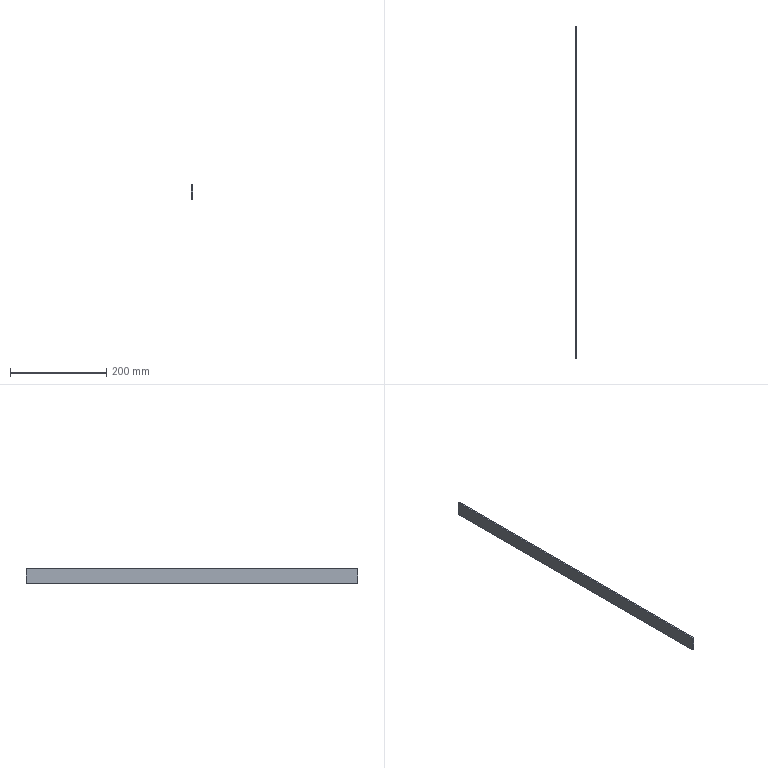Part | SolidWorks | 1 solid | 6 faces | box 3 x 690 x 30 mm | volume 62100 mm3 | plane 6
STEP:
#1=CARTESIAN_POINT('',(0.,345.,15.));
#2=VERTEX_POINT('',#1);
#3=CARTESIAN_POINT('',(0.,-345.,15.));
#4=VERTEX_POINT('',#3);
#5=CARTESIAN_POINT('',(0.,-345.,15.));
#6=DIRECTION('',(0.,-1.,0.));
#7=VECTOR('',#6,1000.);
#8=LINE('',#5,#7);
#9=EDGE_CURVE('',#2,#4,#8,.T.);
#10=ORIENTED_EDGE('',*,*,#9,.F.);
#11=CARTESIAN_POINT('',(-3.,345.,15.));
#12=VERTEX_POINT('',#11);
#13=CARTESIAN_POINT('',(-3.,345.,15.));
#14=DIRECTION('',(1.,0.,0.));
#15=VECTOR('',#14,1000.);
#16=LINE('',#13,#15);
#17=EDGE_CURVE('',#12,#2,#16,.T.);
#18=ORIENTED_EDGE('',*,*,#17,.F.);
#19=CARTESIAN_POINT('',(-3.,-345.,15.));
#20=VERTEX_POINT('',#19);
#21=CARTESIAN_POINT('',(-3.,-345.,15.));
#22=DIRECTION('',(0.,-1.,0.));
#23=VECTOR('',#22,1000.);
#24=LINE('',#21,#23);
#25=EDGE_CURVE('',#12,#20,#24,.T.);
#26=ORIENTED_EDGE('',*,*,#25,.T.);
#27=CARTESIAN_POINT('',(-3.,-345.,15.));
#28=DIRECTION('',(1.,0.,0.));
#29=VECTOR('',#28,1000.);
#30=LINE('',#27,#29);
#31=EDGE_CURVE('',#20,#4,#30,.T.);
#32=ORIENTED_EDGE('',*,*,#31,.T.);
#33=EDGE_LOOP('',(#10,#18,#26,#32));
#34=FACE_OUTER_BOUND('',#33,.T.);
#35=CARTESIAN_POINT('',(-3.,-345.,15.));
#36=DIRECTION('',(0.,0.,1.));
#37=DIRECTION('',(1.,0.,0.));
#38=AXIS2_PLACEMENT_3D('',#35,#36,#37);
#39=PLANE('',#38);
#40=ADVANCED_FACE('',(#34),#39,.T.);
#41=CARTESIAN_POINT('',(0.,345.,-15.));
#42=VERTEX_POINT('',#41);
#43=CARTESIAN_POINT('',(0.,345.,-15.));
#44=DIRECTION('',(0.,0.,1.));
#45=VECTOR('',#44,1000.);
#46=LINE('',#43,#45);
#47=EDGE_CURVE('',#42,#2,#46,.T.);
#48=ORIENTED_EDGE('',*,*,#47,.F.);
#49=CARTESIAN_POINT('',(-3.,345.,-15.));
#50=VERTEX_POINT('',#49);
#51=CARTESIAN_POINT('',(-3.,345.,-15.));
#52=DIRECTION('',(1.,0.,0.));
#53=VECTOR('',#52,1000.);
#54=LINE('',#51,#53);
#55=EDGE_CURVE('',#50,#42,#54,.T.);
#56=ORIENTED_EDGE('',*,*,#55,.F.);
#57=CARTESIAN_POINT('',(-3.,345.,-15.));
#58=DIRECTION('',(0.,0.,1.));
#59=VECTOR('',#58,1000.);
#60=LINE('',#57,#59);
#61=EDGE_CURVE('',#50,#12,#60,.T.);
#62=ORIENTED_EDGE('',*,*,#61,.T.);
#63=ORIENTED_EDGE('',*,*,#17,.T.);
#64=EDGE_LOOP('',(#48,#56,#62,#63));
#65=FACE_OUTER_BOUND('',#64,.T.);
#66=CARTESIAN_POINT('',(-3.,345.,-15.));
#67=DIRECTION('',(0.,1.,0.));
#68=DIRECTION('',(0.,0.,1.));
#69=AXIS2_PLACEMENT_3D('',#66,#67,#68);
#70=PLANE('',#69);
#71=ADVANCED_FACE('',(#65),#70,.T.);
#72=CARTESIAN_POINT('',(0.,-345.,-15.));
#73=VERTEX_POINT('',#72);
#74=CARTESIAN_POINT('',(0.,-345.,-15.));
#75=DIRECTION('',(0.,1.,0.));
#76=VECTOR('',#75,1000.);
#77=LINE('',#74,#76);
#78=EDGE_CURVE('',#73,#42,#77,.T.);
#79=ORIENTED_EDGE('',*,*,#78,.F.);
#80=CARTESIAN_POINT('',(-3.,-345.,-15.));
#81=VERTEX_POINT('',#80);
#82=CARTESIAN_POINT('',(-3.,-345.,-15.));
#83=DIRECTION('',(1.,0.,0.));
#84=VECTOR('',#83,1000.);
#85=LINE('',#82,#84);
#86=EDGE_CURVE('',#81,#73,#85,.T.);
#87=ORIENTED_EDGE('',*,*,#86,.F.);
#88=CARTESIAN_POINT('',(-3.,-345.,-15.));
#89=DIRECTION('',(0.,1.,0.));
#90=VECTOR('',#89,1000.);
#91=LINE('',#88,#90);
#92=EDGE_CURVE('',#81,#50,#91,.T.);
#93=ORIENTED_EDGE('',*,*,#92,.T.);
#94=ORIENTED_EDGE('',*,*,#55,.T.);
#95=EDGE_LOOP('',(#79,#87,#93,#94));
#96=FACE_OUTER_BOUND('',#95,.T.);
#97=CARTESIAN_POINT('',(-3.,-345.,-15.));
#98=DIRECTION('',(0.,0.,-1.));
#99=DIRECTION('',(-1.,0.,0.));
#100=AXIS2_PLACEMENT_3D('',#97,#98,#99);
#101=PLANE('',#100);
#102=ADVANCED_FACE('',(#96),#101,.T.);
#103=CARTESIAN_POINT('',(0.,-345.,-15.));
#104=DIRECTION('',(0.,0.,-1.));
#105=VECTOR('',#104,1000.);
#106=LINE('',#103,#105);
#107=EDGE_CURVE('',#4,#73,#106,.T.);
#108=ORIENTED_EDGE('',*,*,#107,.F.);
#109=ORIENTED_EDGE('',*,*,#31,.F.);
#110=CARTESIAN_POINT('',(-3.,-345.,-15.));
#111=DIRECTION('',(0.,0.,-1.));
#112=VECTOR('',#111,1000.);
#113=LINE('',#110,#112);
#114=EDGE_CURVE('',#20,#81,#113,.T.);
#115=ORIENTED_EDGE('',*,*,#114,.T.);
#116=ORIENTED_EDGE('',*,*,#86,.T.);
#117=EDGE_LOOP('',(#108,#109,#115,#116));
#118=FACE_OUTER_BOUND('',#117,.T.);
#119=CARTESIAN_POINT('',(-3.,-345.,-15.));
#120=DIRECTION('',(0.,-1.,0.));
#121=DIRECTION('',(0.,0.,-1.));
#122=AXIS2_PLACEMENT_3D('',#119,#120,#121);
#123=PLANE('',#122);
#124=ADVANCED_FACE('',(#118),#123,.T.);
#125=ORIENTED_EDGE('',*,*,#25,.F.);
#126=ORIENTED_EDGE('',*,*,#61,.F.);
#127=ORIENTED_EDGE('',*,*,#92,.F.);
#128=ORIENTED_EDGE('',*,*,#114,.F.);
#129=EDGE_LOOP('',(#125,#126,#127,#128));
#130=FACE_OUTER_BOUND('',#129,.T.);
#131=CARTESIAN_POINT('',(-3.,0.,0.));
#132=DIRECTION('',(1.,0.,0.));
#133=DIRECTION('',(0.,0.,-1.));
#134=AXIS2_PLACEMENT_3D('',#131,#132,#133);
#135=PLANE('',#134);
#136=ADVANCED_FACE('',(#130),#135,.F.);
#137=ORIENTED_EDGE('',*,*,#9,.T.);
#138=ORIENTED_EDGE('',*,*,#107,.T.);
#139=ORIENTED_EDGE('',*,*,#78,.T.);
#140=ORIENTED_EDGE('',*,*,#47,.T.);
#141=EDGE_LOOP('',(#137,#138,#139,#140));
#142=FACE_OUTER_BOUND('',#141,.T.);
#143=CARTESIAN_POINT('',(0.,0.,0.));
#144=DIRECTION('',(1.,0.,0.));
#145=DIRECTION('',(0.,0.,-1.));
#146=AXIS2_PLACEMENT_3D('',#143,#144,#145);
#147=PLANE('',#146);
#148=ADVANCED_FACE('',(#142),#147,.T.);
#149=CLOSED_SHELL('',(#40,#71,#102,#124,#136,#148));
#150=MANIFOLD_SOLID_BREP('',#149);
#151=CARTESIAN_POINT('',(0.,0.,0.));
#152=DIRECTION('',(0.,0.,1.));
#153=DIRECTION('',(1.,0.,0.));
#154=AXIS2_PLACEMENT_3D('',#151,#152,#153);
#155=(LENGTH_UNIT()NAMED_UNIT(*)SI_UNIT(.MILLI.,.METRE.));
#156=UNCERTAINTY_MEASURE_WITH_UNIT(LENGTH_MEASURE(0.00001),#155,'','');
#157=(NAMED_UNIT(*)PLANE_ANGLE_UNIT()SI_UNIT($,.RADIAN.));
#158=(NAMED_UNIT(*)SI_UNIT($,.STERADIAN.)SOLID_ANGLE_UNIT());
#159=(GEOMETRIC_REPRESENTATION_CONTEXT(3)GLOBAL_UNCERTAINTY_ASSIGNED_CONTEXT((#156))GLOBAL_UNIT_ASSIGNED_CONTEXT((#155,#157,#158))REPRESENTATION_CONTEXT('',''));
#160=ADVANCED_BREP_SHAPE_REPRESENTATION('',(#150,#154),#159);